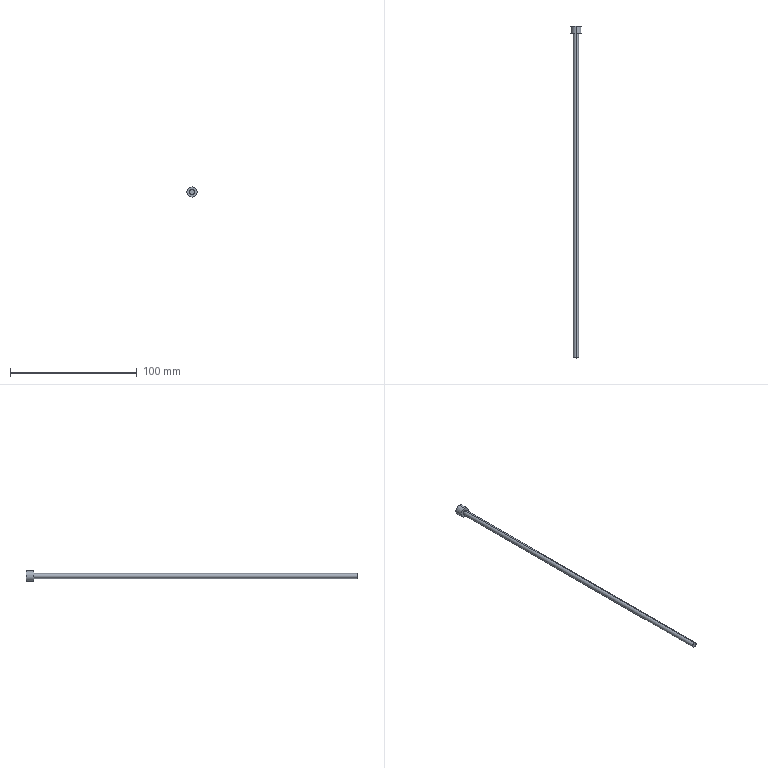Part | STEP file | 1 solid | 7 faces | box 8 x 262.36 x 8 mm | volume 3523 mm3 | cylinder 4 | plane 3 | commonest cylinder face diameters 4 x2 8 x2
STEP:
#1=CARTESIAN_POINT('',(0.,0.,0.));
#2=DIRECTION('',(0.,0.,1.));
#3=DIRECTION('',(1.,0.,0.));
#4=AXIS2_PLACEMENT_3D('',#1,#2,#3);
#5=CARTESIAN_POINT('',(-137.387,290.5,79.529));
#6=VERTEX_POINT('',#5);
#7=CARTESIAN_POINT('',(-137.387,290.5,87.529));
#8=VERTEX_POINT('',#7);
#9=CARTESIAN_POINT('',(-137.387,290.5,83.529));
#10=DIRECTION('',(0.,-1.,0.));
#11=DIRECTION('',(0.,0.,-1.));
#12=AXIS2_PLACEMENT_3D('',#9,#10,#11);
#13=CIRCLE('',#12,4.);
#14=CARTESIAN_POINT('',(-137.387,290.5,83.529));
#15=DIRECTION('',(0.,-1.,0.));
#16=DIRECTION('',(0.,0.,-1.));
#17=AXIS2_PLACEMENT_3D('',#14,#15,#16);
#18=CYLINDRICAL_SURFACE('',#17,4.);
#19=CARTESIAN_POINT('',(0.,0.));
#20=DIRECTION('',(1.,0.));
#21=VECTOR('',#20,1.);
#22=LINE('',#19,#21);
#23=(GEOMETRIC_REPRESENTATION_CONTEXT(2)PARAMETRIC_REPRESENTATION_CONTEXT()REPRESENTATION_CONTEXT('',''));
#24=DEFINITIONAL_REPRESENTATION('',(#22),#23);
#25=PCURVE('',#18,#24);
#26=CARTESIAN_POINT('',(-72.862,290.5,110.196));
#27=DIRECTION('',(0.,-1.,0.));
#28=DIRECTION('',(0.,0.,-1.));
#29=AXIS2_PLACEMENT_3D('',#26,#27,#28);
#30=PLANE('',#29);
#31=CARTESIAN_POINT('',(26.667,-64.524));
#32=DIRECTION('',(1.,0.));
#33=AXIS2_PLACEMENT_2D('',#31,#32);
#34=CIRCLE('',#33,4.);
#35=(GEOMETRIC_REPRESENTATION_CONTEXT(2)PARAMETRIC_REPRESENTATION_CONTEXT()REPRESENTATION_CONTEXT('',''));
#36=DEFINITIONAL_REPRESENTATION('',(#34),#35);
#37=PCURVE('',#30,#36);
#38=SURFACE_CURVE('',#13,(#25,#37),.PCURVE_S1.);
#39=EDGE_CURVE('',#6,#8,#38,.T.);
#40=ORIENTED_EDGE('',*,*,#39,.T.);
#41=CARTESIAN_POINT('',(-137.387,284.5,87.529));
#42=VERTEX_POINT('',#41);
#43=CARTESIAN_POINT('',(-137.387,290.5,87.529));
#44=DIRECTION('',(0.,-1.,0.));
#45=VECTOR('',#44,1.);
#46=LINE('',#43,#45);
#47=CARTESIAN_POINT('',(3.142,0.));
#48=DIRECTION('',(0.,1.));
#49=VECTOR('',#48,1.);
#50=LINE('',#47,#49);
#51=(GEOMETRIC_REPRESENTATION_CONTEXT(2)PARAMETRIC_REPRESENTATION_CONTEXT()REPRESENTATION_CONTEXT('',''));
#52=DEFINITIONAL_REPRESENTATION('',(#50),#51);
#53=PCURVE('',#18,#52);
#54=CARTESIAN_POINT('',(-137.387,290.5,83.529));
#55=DIRECTION('',(0.,-1.,0.));
#56=DIRECTION('',(0.,0.,-1.));
#57=AXIS2_PLACEMENT_3D('',#54,#55,#56);
#58=CYLINDRICAL_SURFACE('',#57,4.);
#59=CARTESIAN_POINT('',(3.142,0.));
#60=DIRECTION('',(0.,1.));
#61=VECTOR('',#60,1.);
#62=LINE('',#59,#61);
#63=(GEOMETRIC_REPRESENTATION_CONTEXT(2)PARAMETRIC_REPRESENTATION_CONTEXT()REPRESENTATION_CONTEXT('',''));
#64=DEFINITIONAL_REPRESENTATION('',(#62),#63);
#65=PCURVE('',#58,#64);
#66=SURFACE_CURVE('',#46,(#53,#65),.PCURVE_S1.);
#67=EDGE_CURVE('',#8,#42,#66,.T.);
#68=ORIENTED_EDGE('',*,*,#67,.T.);
#69=CARTESIAN_POINT('',(-137.387,284.5,79.529));
#70=VERTEX_POINT('',#69);
#71=CARTESIAN_POINT('',(-137.387,284.5,83.529));
#72=DIRECTION('',(0.,1.,0.));
#73=DIRECTION('',(0.,0.,1.));
#74=AXIS2_PLACEMENT_3D('',#71,#72,#73);
#75=CIRCLE('',#74,4.);
#76=CARTESIAN_POINT('',(3.142,6.));
#77=DIRECTION('',(-1.,0.));
#78=VECTOR('',#77,1.);
#79=LINE('',#76,#78);
#80=(GEOMETRIC_REPRESENTATION_CONTEXT(2)PARAMETRIC_REPRESENTATION_CONTEXT()REPRESENTATION_CONTEXT('',''));
#81=DEFINITIONAL_REPRESENTATION('',(#79),#80);
#82=PCURVE('',#18,#81);
#83=CARTESIAN_POINT('',(-137.387,284.5,83.529));
#84=DIRECTION('',(0.,-1.,0.));
#85=DIRECTION('',(0.,0.,-1.));
#86=AXIS2_PLACEMENT_3D('',#83,#84,#85);
#87=PLANE('',#86);
#88=CARTESIAN_POINT('',(-4.,0.));
#89=CARTESIAN_POINT('',(-4.,6.928));
#90=CARTESIAN_POINT('',(2.,3.464));
#91=CARTESIAN_POINT('',(8.,0.));
#92=CARTESIAN_POINT('',(2.,-3.464));
#93=CARTESIAN_POINT('',(-4.,-6.928));
#94=CARTESIAN_POINT('',(-4.,0.));
#95=(BOUNDED_CURVE()B_SPLINE_CURVE(2,(#88,#89,#90,#91,#92,#93,#94),.UNSPECIFIED.,.T.,.F.)B_SPLINE_CURVE_WITH_KNOTS((1,2,2,2,2,1),(-2.094,0.,2.094,4.189,6.283,8.378),.UNSPECIFIED.)CURVE()GEOMETRIC_REPRESENTATION_ITEM()RATIONAL_B_SPLINE_CURVE((1.,0.5,1.,0.5,1.,0.5,1.))REPRESENTATION_ITEM(''));
#96=(GEOMETRIC_REPRESENTATION_CONTEXT(2)PARAMETRIC_REPRESENTATION_CONTEXT()REPRESENTATION_CONTEXT('',''));
#97=DEFINITIONAL_REPRESENTATION('',(#95),#96);
#98=PCURVE('',#87,#97);
#99=SURFACE_CURVE('',#75,(#82,#98),.PCURVE_S1.);
#100=EDGE_CURVE('',#42,#70,#99,.T.);
#101=ORIENTED_EDGE('',*,*,#100,.T.);
#102=CARTESIAN_POINT('',(-137.387,290.5,79.529));
#103=DIRECTION('',(0.,-1.,0.));
#104=VECTOR('',#103,1.);
#105=LINE('',#102,#104);
#106=CARTESIAN_POINT('',(0.,0.));
#107=DIRECTION('',(0.,1.));
#108=VECTOR('',#107,1.);
#109=LINE('',#106,#108);
#110=(GEOMETRIC_REPRESENTATION_CONTEXT(2)PARAMETRIC_REPRESENTATION_CONTEXT()REPRESENTATION_CONTEXT('',''));
#111=DEFINITIONAL_REPRESENTATION('',(#109),#110);
#112=PCURVE('',#18,#111);
#113=CARTESIAN_POINT('',(6.283,0.));
#114=DIRECTION('',(0.,1.));
#115=VECTOR('',#114,1.);
#116=LINE('',#113,#115);
#117=(GEOMETRIC_REPRESENTATION_CONTEXT(2)PARAMETRIC_REPRESENTATION_CONTEXT()REPRESENTATION_CONTEXT('',''));
#118=DEFINITIONAL_REPRESENTATION('',(#116),#117);
#119=PCURVE('',#58,#118);
#120=SURFACE_CURVE('',#105,(#112,#119),.PCURVE_S1.);
#121=EDGE_CURVE('',#6,#70,#120,.T.);
#122=ORIENTED_EDGE('',*,*,#121,.F.);
#123=EDGE_LOOP('',(#40,#68,#101,#122));
#124=FACE_BOUND('',#123,.T.);
#125=ADVANCED_FACE('',(#124),#18,.T.);
#126=CARTESIAN_POINT('',(-137.387,284.5,85.529));
#127=VERTEX_POINT('',#126);
#128=CARTESIAN_POINT('',(-137.387,284.5,81.529));
#129=VERTEX_POINT('',#128);
#130=CARTESIAN_POINT('',(-137.387,284.5,83.529));
#131=DIRECTION('',(0.,1.,0.));
#132=DIRECTION('',(0.,0.,-1.));
#133=AXIS2_PLACEMENT_3D('',#130,#131,#132);
#134=CIRCLE('',#133,2.);
#135=CARTESIAN_POINT('',(-137.387,220.5,83.529));
#136=DIRECTION('',(0.,-1.,0.));
#137=DIRECTION('',(0.,0.,-1.));
#138=AXIS2_PLACEMENT_3D('',#135,#136,#137);
#139=CYLINDRICAL_SURFACE('',#138,2.);
#140=CARTESIAN_POINT('',(6.283,-64.));
#141=DIRECTION('',(-1.,0.));
#142=VECTOR('',#141,1.);
#143=LINE('',#140,#142);
#144=(GEOMETRIC_REPRESENTATION_CONTEXT(2)PARAMETRIC_REPRESENTATION_CONTEXT()REPRESENTATION_CONTEXT('',''));
#145=DEFINITIONAL_REPRESENTATION('',(#143),#144);
#146=PCURVE('',#139,#145);
#147=CARTESIAN_POINT('',(2.,0.));
#148=CARTESIAN_POINT('',(2.,-3.464));
#149=CARTESIAN_POINT('',(-1.,-1.732));
#150=CARTESIAN_POINT('',(-4.,0.));
#151=CARTESIAN_POINT('',(-1.,1.732));
#152=CARTESIAN_POINT('',(2.,3.464));
#153=CARTESIAN_POINT('',(2.,0.));
#154=(BOUNDED_CURVE()B_SPLINE_CURVE(2,(#147,#148,#149,#150,#151,#152,#153),.UNSPECIFIED.,.T.,.F.)B_SPLINE_CURVE_WITH_KNOTS((1,2,2,2,2,1),(-2.094,0.,2.094,4.189,6.283,8.378),.UNSPECIFIED.)CURVE()GEOMETRIC_REPRESENTATION_ITEM()RATIONAL_B_SPLINE_CURVE((1.,0.5,1.,0.5,1.,0.5,1.))REPRESENTATION_ITEM(''));
#155=(GEOMETRIC_REPRESENTATION_CONTEXT(2)PARAMETRIC_REPRESENTATION_CONTEXT()REPRESENTATION_CONTEXT('',''));
#156=DEFINITIONAL_REPRESENTATION('',(#154),#155);
#157=PCURVE('',#87,#156);
#158=SURFACE_CURVE('',#134,(#146,#157),.PCURVE_S1.);
#159=EDGE_CURVE('',#127,#129,#158,.T.);
#160=ORIENTED_EDGE('',*,*,#159,.F.);
#161=CARTESIAN_POINT('',(-137.387,28.14,85.529));
#162=VERTEX_POINT('',#161);
#163=CARTESIAN_POINT('',(-137.387,220.5,85.529));
#164=DIRECTION('',(0.,-1.,0.));
#165=VECTOR('',#164,1.);
#166=LINE('',#163,#165);
#167=CARTESIAN_POINT('',(3.142,0.));
#168=DIRECTION('',(0.,1.));
#169=VECTOR('',#168,1.);
#170=LINE('',#167,#169);
#171=(GEOMETRIC_REPRESENTATION_CONTEXT(2)PARAMETRIC_REPRESENTATION_CONTEXT()REPRESENTATION_CONTEXT('',''));
#172=DEFINITIONAL_REPRESENTATION('',(#170),#171);
#173=PCURVE('',#139,#172);
#174=CARTESIAN_POINT('',(-137.387,220.5,83.529));
#175=DIRECTION('',(0.,-1.,0.));
#176=DIRECTION('',(0.,0.,-1.));
#177=AXIS2_PLACEMENT_3D('',#174,#175,#176);
#178=CYLINDRICAL_SURFACE('',#177,2.);
#179=CARTESIAN_POINT('',(3.142,0.));
#180=DIRECTION('',(0.,1.));
#181=VECTOR('',#180,1.);
#182=LINE('',#179,#181);
#183=(GEOMETRIC_REPRESENTATION_CONTEXT(2)PARAMETRIC_REPRESENTATION_CONTEXT()REPRESENTATION_CONTEXT('',''));
#184=DEFINITIONAL_REPRESENTATION('',(#182),#183);
#185=PCURVE('',#178,#184);
#186=SURFACE_CURVE('',#166,(#173,#185),.PCURVE_S1.);
#187=EDGE_CURVE('',#127,#162,#186,.T.);
#188=ORIENTED_EDGE('',*,*,#187,.T.);
#189=CARTESIAN_POINT('',(-137.387,28.14,81.529));
#190=VERTEX_POINT('',#189);
#191=CARTESIAN_POINT('',(-137.387,28.14,83.529));
#192=DIRECTION('',(0.,1.,0.));
#193=DIRECTION('',(0.,0.,-1.));
#194=AXIS2_PLACEMENT_3D('',#191,#192,#193);
#195=CIRCLE('',#194,2.);
#196=CARTESIAN_POINT('',(6.283,192.36));
#197=DIRECTION('',(-1.,0.));
#198=VECTOR('',#197,1.);
#199=LINE('',#196,#198);
#200=(GEOMETRIC_REPRESENTATION_CONTEXT(2)PARAMETRIC_REPRESENTATION_CONTEXT()REPRESENTATION_CONTEXT('',''));
#201=DEFINITIONAL_REPRESENTATION('',(#199),#200);
#202=PCURVE('',#139,#201);
#203=CARTESIAN_POINT('',(-72.862,28.14,-91.563));
#204=DIRECTION('',(0.,-1.,0.));
#205=DIRECTION('',(0.,0.,-1.));
#206=AXIS2_PLACEMENT_3D('',#203,#204,#205);
#207=PLANE('',#206);
#208=CARTESIAN_POINT('',(-173.092,-64.524));
#209=CARTESIAN_POINT('',(-173.092,-67.988));
#210=CARTESIAN_POINT('',(-176.092,-66.256));
#211=CARTESIAN_POINT('',(-179.092,-64.524));
#212=CARTESIAN_POINT('',(-176.092,-62.792));
#213=CARTESIAN_POINT('',(-173.092,-61.06));
#214=CARTESIAN_POINT('',(-173.092,-64.524));
#215=(BOUNDED_CURVE()B_SPLINE_CURVE(2,(#208,#209,#210,#211,#212,#213,#214),.UNSPECIFIED.,.T.,.F.)B_SPLINE_CURVE_WITH_KNOTS((1,2,2,2,2,1),(-2.094,0.,2.094,4.189,6.283,8.378),.UNSPECIFIED.)CURVE()GEOMETRIC_REPRESENTATION_ITEM()RATIONAL_B_SPLINE_CURVE((1.,0.5,1.,0.5,1.,0.5,1.))REPRESENTATION_ITEM(''));
#216=(GEOMETRIC_REPRESENTATION_CONTEXT(2)PARAMETRIC_REPRESENTATION_CONTEXT()REPRESENTATION_CONTEXT('',''));
#217=DEFINITIONAL_REPRESENTATION('',(#215),#216);
#218=PCURVE('',#207,#217);
#219=SURFACE_CURVE('',#195,(#202,#218),.PCURVE_S1.);
#220=EDGE_CURVE('',#162,#190,#219,.T.);
#221=ORIENTED_EDGE('',*,*,#220,.T.);
#222=CARTESIAN_POINT('',(-137.387,220.5,81.529));
#223=DIRECTION('',(0.,-1.,0.));
#224=VECTOR('',#223,1.);
#225=LINE('',#222,#224);
#226=CARTESIAN_POINT('',(0.,0.));
#227=DIRECTION('',(0.,1.));
#228=VECTOR('',#227,1.);
#229=LINE('',#226,#228);
#230=(GEOMETRIC_REPRESENTATION_CONTEXT(2)PARAMETRIC_REPRESENTATION_CONTEXT()REPRESENTATION_CONTEXT('',''));
#231=DEFINITIONAL_REPRESENTATION('',(#229),#230);
#232=PCURVE('',#139,#231);
#233=CARTESIAN_POINT('',(6.283,0.));
#234=DIRECTION('',(0.,1.));
#235=VECTOR('',#234,1.);
#236=LINE('',#233,#235);
#237=(GEOMETRIC_REPRESENTATION_CONTEXT(2)PARAMETRIC_REPRESENTATION_CONTEXT()REPRESENTATION_CONTEXT('',''));
#238=DEFINITIONAL_REPRESENTATION('',(#236),#237);
#239=PCURVE('',#178,#238);
#240=SURFACE_CURVE('',#225,(#232,#239),.PCURVE_S1.);
#241=EDGE_CURVE('',#129,#190,#240,.T.);
#242=ORIENTED_EDGE('',*,*,#241,.F.);
#243=EDGE_LOOP('',(#160,#188,#221,#242));
#244=FACE_BOUND('',#243,.T.);
#245=ADVANCED_FACE('',(#244),#139,.T.);
#246=ORIENTED_EDGE('',*,*,#187,.F.);
#247=CARTESIAN_POINT('',(-137.387,284.5,83.529));
#248=DIRECTION('',(0.,1.,0.));
#249=DIRECTION('',(0.,0.,-1.));
#250=AXIS2_PLACEMENT_3D('',#247,#248,#249);
#251=CIRCLE('',#250,2.);
#252=CARTESIAN_POINT('',(6.283,-64.));
#253=DIRECTION('',(-1.,0.));
#254=VECTOR('',#253,1.);
#255=LINE('',#252,#254);
#256=(GEOMETRIC_REPRESENTATION_CONTEXT(2)PARAMETRIC_REPRESENTATION_CONTEXT()REPRESENTATION_CONTEXT('',''));
#257=DEFINITIONAL_REPRESENTATION('',(#255),#256);
#258=PCURVE('',#178,#257);
#259=CARTESIAN_POINT('',(2.,0.));
#260=CARTESIAN_POINT('',(2.,-3.464));
#261=CARTESIAN_POINT('',(-1.,-1.732));
#262=CARTESIAN_POINT('',(-4.,0.));
#263=CARTESIAN_POINT('',(-1.,1.732));
#264=CARTESIAN_POINT('',(2.,3.464));
#265=CARTESIAN_POINT('',(2.,0.));
#266=(BOUNDED_CURVE()B_SPLINE_CURVE(2,(#259,#260,#261,#262,#263,#264,#265),.UNSPECIFIED.,.T.,.F.)B_SPLINE_CURVE_WITH_KNOTS((1,2,2,2,2,1),(-2.094,0.,2.094,4.189,6.283,8.378),.UNSPECIFIED.)CURVE()GEOMETRIC_REPRESENTATION_ITEM()RATIONAL_B_SPLINE_CURVE((1.,0.5,1.,0.5,1.,0.5,1.))REPRESENTATION_ITEM(''));
#267=(GEOMETRIC_REPRESENTATION_CONTEXT(2)PARAMETRIC_REPRESENTATION_CONTEXT()REPRESENTATION_CONTEXT('',''));
#268=DEFINITIONAL_REPRESENTATION('',(#266),#267);
#269=PCURVE('',#87,#268);
#270=SURFACE_CURVE('',#251,(#258,#269),.PCURVE_S1.);
#271=EDGE_CURVE('',#129,#127,#270,.T.);
#272=ORIENTED_EDGE('',*,*,#271,.F.);
#273=ORIENTED_EDGE('',*,*,#241,.T.);
#274=CARTESIAN_POINT('',(-137.387,28.14,83.529));
#275=DIRECTION('',(0.,1.,0.));
#276=DIRECTION('',(0.,0.,-1.));
#277=AXIS2_PLACEMENT_3D('',#274,#275,#276);
#278=CIRCLE('',#277,2.);
#279=CARTESIAN_POINT('',(6.283,192.36));
#280=DIRECTION('',(-1.,0.));
#281=VECTOR('',#280,1.);
#282=LINE('',#279,#281);
#283=(GEOMETRIC_REPRESENTATION_CONTEXT(2)PARAMETRIC_REPRESENTATION_CONTEXT()REPRESENTATION_CONTEXT('',''));
#284=DEFINITIONAL_REPRESENTATION('',(#282),#283);
#285=PCURVE('',#178,#284);
#286=CARTESIAN_POINT('',(-173.092,-64.524));
#287=CARTESIAN_POINT('',(-173.092,-67.988));
#288=CARTESIAN_POINT('',(-176.092,-66.256));
#289=CARTESIAN_POINT('',(-179.092,-64.524));
#290=CARTESIAN_POINT('',(-176.092,-62.792));
#291=CARTESIAN_POINT('',(-173.092,-61.06));
#292=CARTESIAN_POINT('',(-173.092,-64.524));
#293=(BOUNDED_CURVE()B_SPLINE_CURVE(2,(#286,#287,#288,#289,#290,#291,#292),.UNSPECIFIED.,.T.,.F.)B_SPLINE_CURVE_WITH_KNOTS((1,2,2,2,2,1),(-2.094,0.,2.094,4.189,6.283,8.378),.UNSPECIFIED.)CURVE()GEOMETRIC_REPRESENTATION_ITEM()RATIONAL_B_SPLINE_CURVE((1.,0.5,1.,0.5,1.,0.5,1.))REPRESENTATION_ITEM(''));
#294=(GEOMETRIC_REPRESENTATION_CONTEXT(2)PARAMETRIC_REPRESENTATION_CONTEXT()REPRESENTATION_CONTEXT('',''));
#295=DEFINITIONAL_REPRESENTATION('',(#293),#294);
#296=PCURVE('',#207,#295);
#297=SURFACE_CURVE('',#278,(#285,#296),.PCURVE_S1.);
#298=EDGE_CURVE('',#190,#162,#297,.T.);
#299=ORIENTED_EDGE('',*,*,#298,.T.);
#300=EDGE_LOOP('',(#246,#272,#273,#299));
#301=FACE_BOUND('',#300,.T.);
#302=ADVANCED_FACE('',(#301),#178,.T.);
#303=ORIENTED_EDGE('',*,*,#298,.F.);
#304=ORIENTED_EDGE('',*,*,#220,.F.);
#305=EDGE_LOOP('',(#303,#304));
#306=FACE_BOUND('',#305,.T.);
#307=ADVANCED_FACE('',(#306),#207,.T.);
#308=ORIENTED_EDGE('',*,*,#271,.T.);
#309=ORIENTED_EDGE('',*,*,#159,.T.);
#310=EDGE_LOOP('',(#308,#309));
#311=FACE_BOUND('',#310,.T.);
#312=CARTESIAN_POINT('',(-137.387,284.5,83.529));
#313=DIRECTION('',(0.,1.,0.));
#314=DIRECTION('',(0.,0.,1.));
#315=AXIS2_PLACEMENT_3D('',#312,#313,#314);
#316=CIRCLE('',#315,4.);
#317=CARTESIAN_POINT('',(-4.,0.));
#318=CARTESIAN_POINT('',(-4.,6.928));
#319=CARTESIAN_POINT('',(2.,3.464));
#320=CARTESIAN_POINT('',(8.,0.));
#321=CARTESIAN_POINT('',(2.,-3.464));
#322=CARTESIAN_POINT('',(-4.,-6.928));
#323=CARTESIAN_POINT('',(-4.,0.));
#324=(BOUNDED_CURVE()B_SPLINE_CURVE(2,(#317,#318,#319,#320,#321,#322,#323),.UNSPECIFIED.,.T.,.F.)B_SPLINE_CURVE_WITH_KNOTS((1,2,2,2,2,1),(-2.094,0.,2.094,4.189,6.283,8.378),.UNSPECIFIED.)CURVE()GEOMETRIC_REPRESENTATION_ITEM()RATIONAL_B_SPLINE_CURVE((1.,0.5,1.,0.5,1.,0.5,1.))REPRESENTATION_ITEM(''));
#325=(GEOMETRIC_REPRESENTATION_CONTEXT(2)PARAMETRIC_REPRESENTATION_CONTEXT()REPRESENTATION_CONTEXT('',''));
#326=DEFINITIONAL_REPRESENTATION('',(#324),#325);
#327=PCURVE('',#87,#326);
#328=CARTESIAN_POINT('',(9.425,6.));
#329=DIRECTION('',(-1.,0.));
#330=VECTOR('',#329,1.);
#331=LINE('',#328,#330);
#332=(GEOMETRIC_REPRESENTATION_CONTEXT(2)PARAMETRIC_REPRESENTATION_CONTEXT()REPRESENTATION_CONTEXT('',''));
#333=DEFINITIONAL_REPRESENTATION('',(#331),#332);
#334=PCURVE('',#58,#333);
#335=SURFACE_CURVE('',#316,(#327,#334),.PCURVE_S1.);
#336=EDGE_CURVE('',#70,#42,#335,.T.);
#337=ORIENTED_EDGE('',*,*,#336,.F.);
#338=ORIENTED_EDGE('',*,*,#100,.F.);
#339=EDGE_LOOP('',(#337,#338));
#340=FACE_BOUND('',#339,.T.);
#341=ADVANCED_FACE('',(#311,#340),#87,.T.);
#342=ORIENTED_EDGE('',*,*,#67,.F.);
#343=CARTESIAN_POINT('',(-137.387,290.5,83.529));
#344=DIRECTION('',(0.,-1.,0.));
#345=DIRECTION('',(0.,0.,-1.));
#346=AXIS2_PLACEMENT_3D('',#343,#344,#345);
#347=CIRCLE('',#346,4.);
#348=CARTESIAN_POINT('',(0.,0.));
#349=DIRECTION('',(1.,0.));
#350=VECTOR('',#349,1.);
#351=LINE('',#348,#350);
#352=(GEOMETRIC_REPRESENTATION_CONTEXT(2)PARAMETRIC_REPRESENTATION_CONTEXT()REPRESENTATION_CONTEXT('',''));
#353=DEFINITIONAL_REPRESENTATION('',(#351),#352);
#354=PCURVE('',#58,#353);
#355=CARTESIAN_POINT('',(26.667,-64.524));
#356=DIRECTION('',(1.,0.));
#357=AXIS2_PLACEMENT_2D('',#355,#356);
#358=CIRCLE('',#357,4.);
#359=(GEOMETRIC_REPRESENTATION_CONTEXT(2)PARAMETRIC_REPRESENTATION_CONTEXT()REPRESENTATION_CONTEXT('',''));
#360=DEFINITIONAL_REPRESENTATION('',(#358),#359);
#361=PCURVE('',#30,#360);
#362=SURFACE_CURVE('',#347,(#354,#361),.PCURVE_S1.);
#363=EDGE_CURVE('',#8,#6,#362,.T.);
#364=ORIENTED_EDGE('',*,*,#363,.T.);
#365=ORIENTED_EDGE('',*,*,#121,.T.);
#366=ORIENTED_EDGE('',*,*,#336,.T.);
#367=EDGE_LOOP('',(#342,#364,#365,#366));
#368=FACE_BOUND('',#367,.T.);
#369=ADVANCED_FACE('',(#368),#58,.T.);
#370=ORIENTED_EDGE('',*,*,#39,.F.);
#371=ORIENTED_EDGE('',*,*,#363,.F.);
#372=EDGE_LOOP('',(#370,#371));
#373=FACE_BOUND('',#372,.T.);
#374=ADVANCED_FACE('',(#373),#30,.F.);
#375=CLOSED_SHELL('',(#125,#245,#302,#307,#341,#369,#374));
#376=MANIFOLD_SOLID_BREP('',#375);
#377=(LENGTH_UNIT()NAMED_UNIT(*)SI_UNIT(.MILLI.,.METRE.));
#378=UNCERTAINTY_MEASURE_WITH_UNIT(LENGTH_MEASURE(0.0000001),#377,'','');
#379=(NAMED_UNIT(*)PLANE_ANGLE_UNIT()SI_UNIT($,.RADIAN.));
#380=(NAMED_UNIT(*)SI_UNIT($,.STERADIAN.)SOLID_ANGLE_UNIT());
#381=(GEOMETRIC_REPRESENTATION_CONTEXT(3)GLOBAL_UNCERTAINTY_ASSIGNED_CONTEXT((#378))GLOBAL_UNIT_ASSIGNED_CONTEXT((#377,#379,#380))REPRESENTATION_CONTEXT('',''));
#382=ADVANCED_BREP_SHAPE_REPRESENTATION('',(#4,#376),#381);